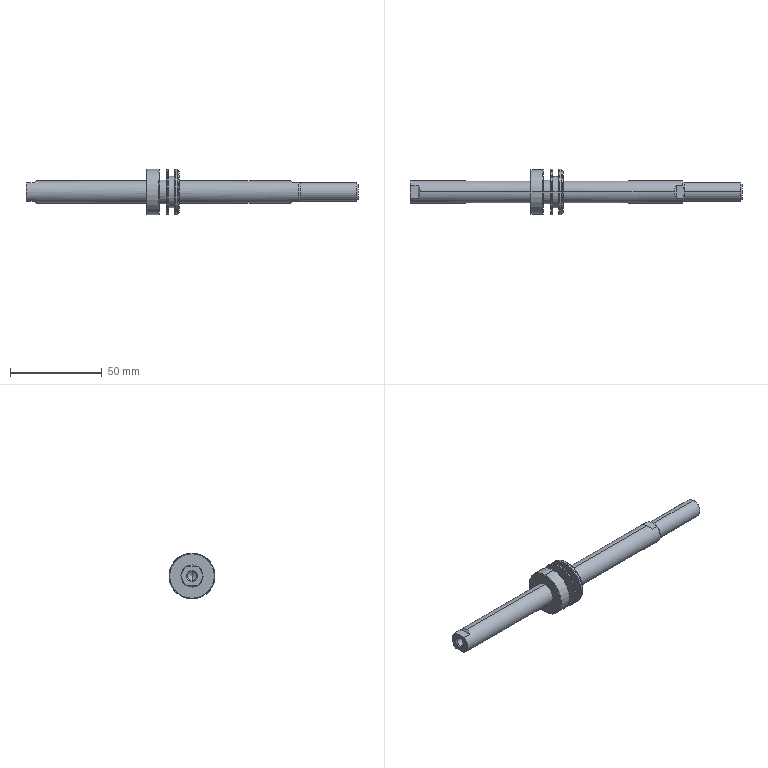Part | STEP file | ACQJ25x50-10S-02-cc | 1 solid | 61 faces | box 180.5 x 25 x 25 mm | volume 23193 mm3 | cylinder 20 | plane 17 | cone 16 | spline 8 | commonest cylinder face diameters 12 x4 25 x4 4.917 x2 10 x2 13 x2 17 x2